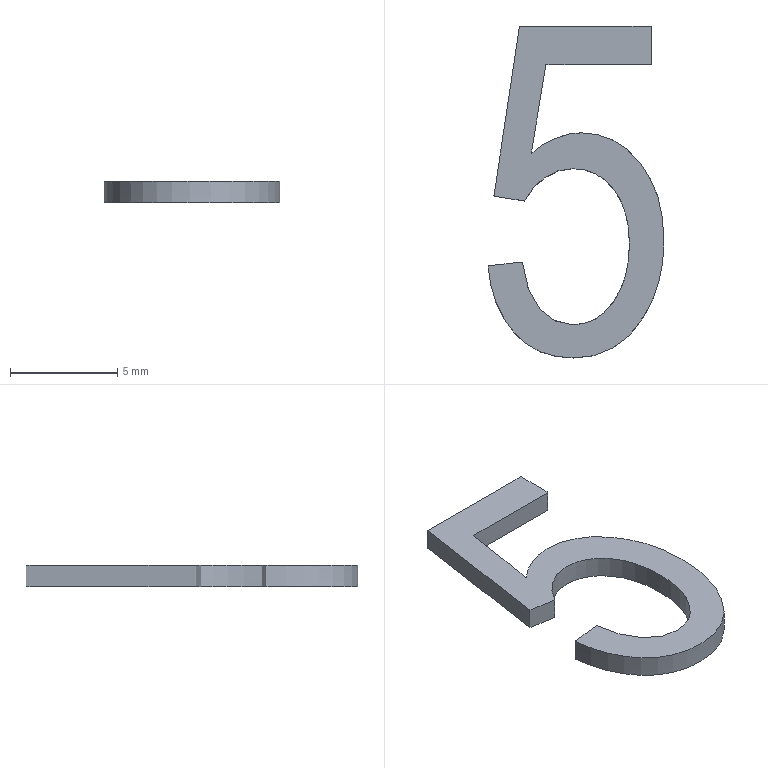Part | STEP file | lll_id1490_x_t | 1 solid | 3 faces | box 8.189 x 15.465 x 1 mm | volume 45.656 mm3 | plane 2 | other 1